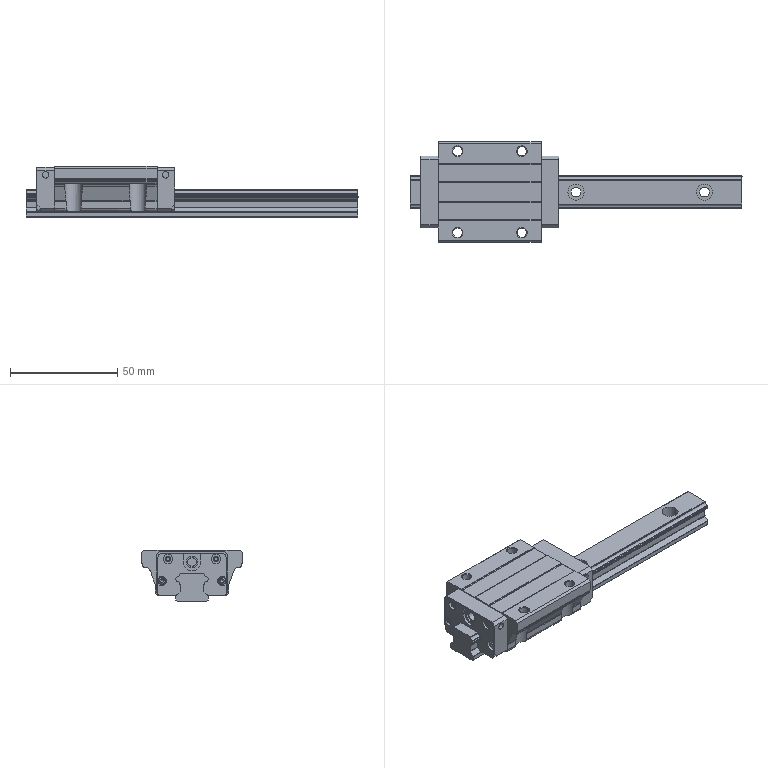Part | STEP file | SHS15C-1SS-155 | 6 solids | 548 faces | box 155 x 47 x 24.001 mm | volume 62079 mm3 | plane 347 | cylinder 161 | spline 32 | cone 8 | commonest cylinder face diameters 4 x22 0.6 x18 1 x12 4.5 x11 3 x10 2 x9